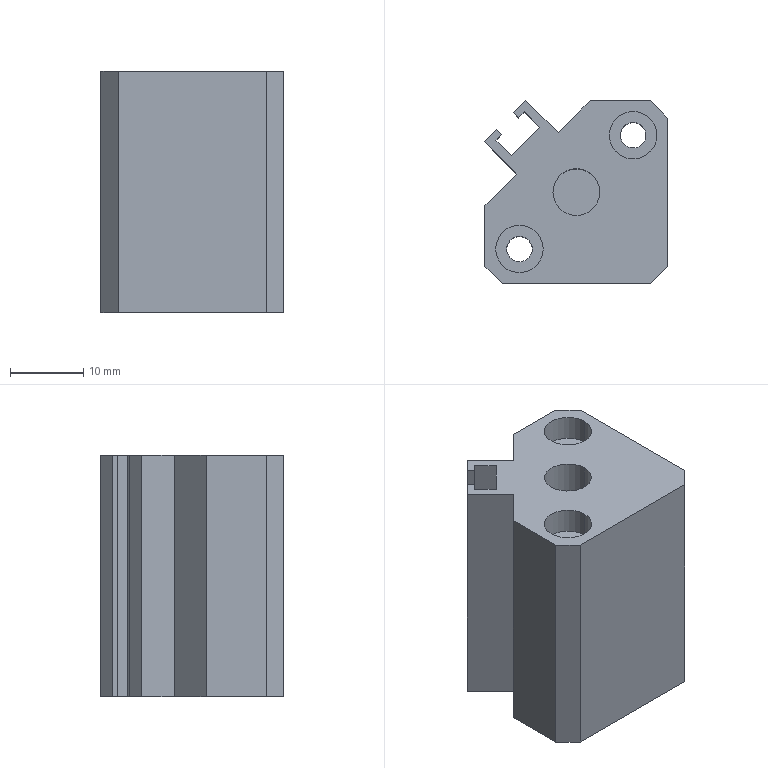Part | STEP file | 3 | 1 solid | 51 faces | box 25.087 x 25.087 x 33 mm | volume 16395 mm3 | plane 29 | cylinder 18 | cone 4 | commonest cylinder face diameters 6.5 x8 3.5 x4 4.13 x4 6.4 x2